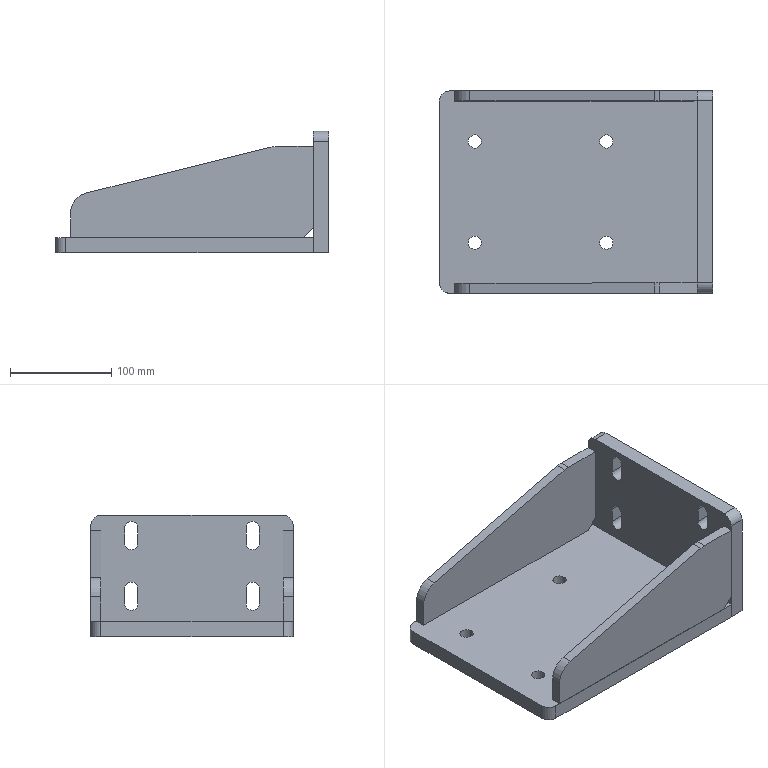Part | SolidWorks | features BaseBody 4 | 4 solids | 64 faces | box 270 x 200 x 120 mm | volume 1426137 mm3 | plane 36 | cylinder 28 | commonest cylinder face diameters 13 x20 20 x4 40 x4